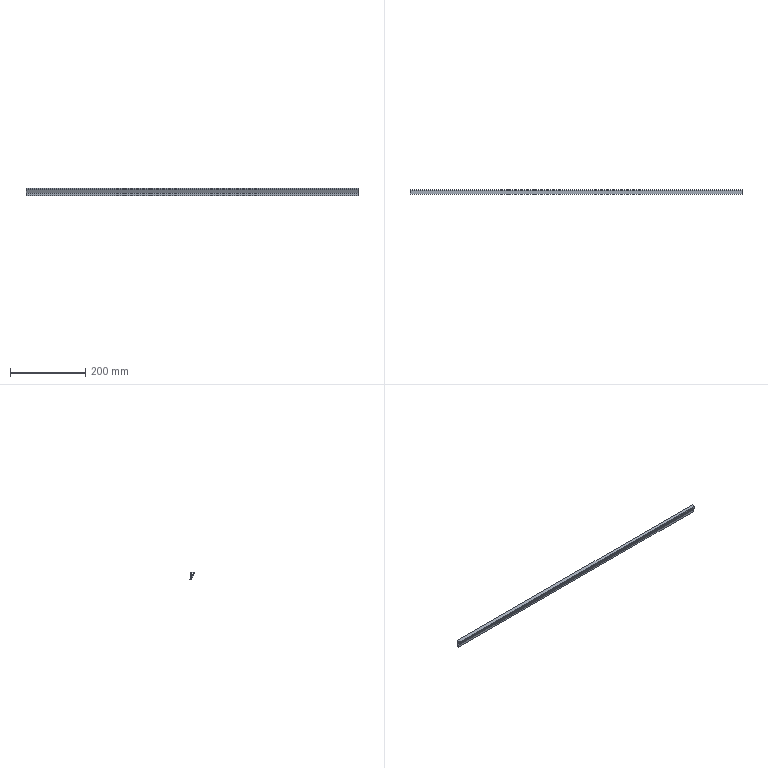Part | SolidWorks | features BaseBody 1 | 1 solid | 13 faces | box 880 x 12 x 21 mm | volume 96538 mm3 | plane 13
STEP:
#1=CARTESIAN_POINT('',(440.,0.,0.));
#2=VERTEX_POINT('',#1);
#3=CARTESIAN_POINT('',(-440.,0.,0.));
#4=VERTEX_POINT('',#3);
#5=CARTESIAN_POINT('',(440.,0.,0.));
#6=DIRECTION('',(-1.,0.,0.));
#7=VECTOR('',#6,1000.);
#8=LINE('',#5,#7);
#9=EDGE_CURVE('',#2,#4,#8,.T.);
#10=ORIENTED_EDGE('',*,*,#9,.F.);
#11=CARTESIAN_POINT('',(440.,0.,-19.));
#12=VERTEX_POINT('',#11);
#13=CARTESIAN_POINT('',(440.,0.,-19.));
#14=DIRECTION('',(0.,0.,1.));
#15=VECTOR('',#14,1000.);
#16=LINE('',#13,#15);
#17=EDGE_CURVE('',#12,#2,#16,.T.);
#18=ORIENTED_EDGE('',*,*,#17,.F.);
#19=CARTESIAN_POINT('',(-440.,0.,-19.));
#20=VERTEX_POINT('',#19);
#21=CARTESIAN_POINT('',(440.,0.,-19.));
#22=DIRECTION('',(1.,0.,0.));
#23=VECTOR('',#22,1000.);
#24=LINE('',#21,#23);
#25=EDGE_CURVE('',#20,#12,#24,.T.);
#26=ORIENTED_EDGE('',*,*,#25,.F.);
#27=CARTESIAN_POINT('',(-440.,0.,-19.));
#28=DIRECTION('',(0.,0.,-1.));
#29=VECTOR('',#28,1000.);
#30=LINE('',#27,#29);
#31=EDGE_CURVE('',#4,#20,#30,.T.);
#32=ORIENTED_EDGE('',*,*,#31,.F.);
#33=EDGE_LOOP('',(#10,#18,#26,#32));
#34=FACE_OUTER_BOUND('',#33,.T.);
#35=CARTESIAN_POINT('',(440.,0.,-19.));
#36=DIRECTION('',(0.,-1.,0.));
#37=DIRECTION('',(0.,0.,-1.));
#38=AXIS2_PLACEMENT_3D('',#35,#36,#37);
#39=PLANE('',#38);
#40=ADVANCED_FACE('',(#34),#39,.F.);
#41=CARTESIAN_POINT('',(-440.,-3.,-3.));
#42=VERTEX_POINT('',#41);
#43=CARTESIAN_POINT('',(-440.,-3.,-21.));
#44=VERTEX_POINT('',#43);
#45=CARTESIAN_POINT('',(-440.,-3.,0.));
#46=DIRECTION('',(0.,0.,-1.));
#47=VECTOR('',#46,1000.);
#48=LINE('',#45,#47);
#49=EDGE_CURVE('',#42,#44,#48,.T.);
#50=ORIENTED_EDGE('',*,*,#49,.F.);
#51=CARTESIAN_POINT('',(-440.,-7.,-3.));
#52=VERTEX_POINT('',#51);
#53=CARTESIAN_POINT('',(-440.,0.,-3.));
#54=DIRECTION('',(0.,1.,0.));
#55=VECTOR('',#54,1000.);
#56=LINE('',#53,#55);
#57=EDGE_CURVE('',#52,#42,#56,.T.);
#58=ORIENTED_EDGE('',*,*,#57,.F.);
#59=CARTESIAN_POINT('',(-440.,-5.,-7.134));
#60=VERTEX_POINT('',#59);
#61=CARTESIAN_POINT('',(-440.,-5.,-7.134));
#62=DIRECTION('',(0.,-0.4355,0.9002));
#63=VECTOR('',#62,1000.);
#64=LINE('',#61,#63);
#65=EDGE_CURVE('',#60,#52,#64,.T.);
#66=ORIENTED_EDGE('',*,*,#65,.F.);
#67=CARTESIAN_POINT('',(-440.,-5.,-13.334));
#68=VERTEX_POINT('',#67);
#69=CARTESIAN_POINT('',(-440.,-5.,0.));
#70=DIRECTION('',(0.,0.,1.));
#71=VECTOR('',#70,1000.);
#72=LINE('',#69,#71);
#73=EDGE_CURVE('',#68,#60,#72,.T.);
#74=ORIENTED_EDGE('',*,*,#73,.F.);
#75=CARTESIAN_POINT('',(-440.,-10.,-3.));
#76=VERTEX_POINT('',#75);
#77=CARTESIAN_POINT('',(-440.,-10.,-3.));
#78=DIRECTION('',(0.,0.4355,-0.9002));
#79=VECTOR('',#78,1000.);
#80=LINE('',#77,#79);
#81=EDGE_CURVE('',#76,#68,#80,.T.);
#82=ORIENTED_EDGE('',*,*,#81,.F.);
#83=CARTESIAN_POINT('',(-440.,-10.,0.));
#84=VERTEX_POINT('',#83);
#85=CARTESIAN_POINT('',(-440.,-10.,0.));
#86=DIRECTION('',(0.,0.,-1.));
#87=VECTOR('',#86,1000.);
#88=LINE('',#85,#87);
#89=EDGE_CURVE('',#84,#76,#88,.T.);
#90=ORIENTED_EDGE('',*,*,#89,.F.);
#91=CARTESIAN_POINT('',(-440.,0.,0.));
#92=DIRECTION('',(0.,-1.,0.));
#93=VECTOR('',#92,1000.);
#94=LINE('',#91,#93);
#95=EDGE_CURVE('',#4,#84,#94,.T.);
#96=ORIENTED_EDGE('',*,*,#95,.F.);
#97=ORIENTED_EDGE('',*,*,#31,.T.);
#98=CARTESIAN_POINT('',(-440.,2.,-19.));
#99=VERTEX_POINT('',#98);
#100=CARTESIAN_POINT('',(-440.,0.,-19.));
#101=DIRECTION('',(0.,-1.,0.));
#102=VECTOR('',#101,1000.);
#103=LINE('',#100,#102);
#104=EDGE_CURVE('',#99,#20,#103,.T.);
#105=ORIENTED_EDGE('',*,*,#104,.F.);
#106=CARTESIAN_POINT('',(-440.,2.,-21.));
#107=VERTEX_POINT('',#106);
#108=CARTESIAN_POINT('',(-440.,2.,0.));
#109=DIRECTION('',(0.,0.,1.));
#110=VECTOR('',#109,1000.);
#111=LINE('',#108,#110);
#112=EDGE_CURVE('',#107,#99,#111,.T.);
#113=ORIENTED_EDGE('',*,*,#112,.F.);
#114=CARTESIAN_POINT('',(-440.,0.,-21.));
#115=DIRECTION('',(0.,1.,0.));
#116=VECTOR('',#115,1000.);
#117=LINE('',#114,#116);
#118=EDGE_CURVE('',#44,#107,#117,.T.);
#119=ORIENTED_EDGE('',*,*,#118,.F.);
#120=EDGE_LOOP('',(#50,#58,#66,#74,#82,#90,#96,#97,#105,#113,#119));
#121=FACE_OUTER_BOUND('',#120,.T.);
#122=CARTESIAN_POINT('',(-440.,0.,0.));
#123=DIRECTION('',(1.,0.,0.));
#124=DIRECTION('',(0.,0.,-1.));
#125=AXIS2_PLACEMENT_3D('',#122,#123,#124);
#126=PLANE('',#125);
#127=ADVANCED_FACE('',(#121),#126,.F.);
#128=CARTESIAN_POINT('',(440.,-10.,0.));
#129=VERTEX_POINT('',#128);
#130=CARTESIAN_POINT('',(440.,-10.,0.));
#131=DIRECTION('',(-1.,0.,0.));
#132=VECTOR('',#131,1000.);
#133=LINE('',#130,#132);
#134=EDGE_CURVE('',#129,#84,#133,.T.);
#135=ORIENTED_EDGE('',*,*,#134,.F.);
#136=CARTESIAN_POINT('',(440.,0.,0.));
#137=DIRECTION('',(0.,-1.,0.));
#138=VECTOR('',#137,1000.);
#139=LINE('',#136,#138);
#140=EDGE_CURVE('',#2,#129,#139,.T.);
#141=ORIENTED_EDGE('',*,*,#140,.F.);
#142=ORIENTED_EDGE('',*,*,#9,.T.);
#143=ORIENTED_EDGE('',*,*,#95,.T.);
#144=EDGE_LOOP('',(#135,#141,#142,#143));
#145=FACE_OUTER_BOUND('',#144,.T.);
#146=CARTESIAN_POINT('',(440.,0.,0.));
#147=DIRECTION('',(0.,0.,-1.));
#148=DIRECTION('',(-1.,0.,0.));
#149=AXIS2_PLACEMENT_3D('',#146,#147,#148);
#150=PLANE('',#149);
#151=ADVANCED_FACE('',(#145),#150,.F.);
#152=CARTESIAN_POINT('',(440.,-7.,-3.));
#153=VERTEX_POINT('',#152);
#154=CARTESIAN_POINT('',(440.,-3.,-3.));
#155=VERTEX_POINT('',#154);
#156=CARTESIAN_POINT('',(440.,0.,-3.));
#157=DIRECTION('',(0.,1.,0.));
#158=VECTOR('',#157,1000.);
#159=LINE('',#156,#158);
#160=EDGE_CURVE('',#153,#155,#159,.T.);
#161=ORIENTED_EDGE('',*,*,#160,.T.);
#162=CARTESIAN_POINT('',(440.,-3.,-21.));
#163=VERTEX_POINT('',#162);
#164=CARTESIAN_POINT('',(440.,-3.,0.));
#165=DIRECTION('',(0.,0.,-1.));
#166=VECTOR('',#165,1000.);
#167=LINE('',#164,#166);
#168=EDGE_CURVE('',#155,#163,#167,.T.);
#169=ORIENTED_EDGE('',*,*,#168,.T.);
#170=CARTESIAN_POINT('',(440.,2.,-21.));
#171=VERTEX_POINT('',#170);
#172=CARTESIAN_POINT('',(440.,0.,-21.));
#173=DIRECTION('',(0.,1.,0.));
#174=VECTOR('',#173,1000.);
#175=LINE('',#172,#174);
#176=EDGE_CURVE('',#163,#171,#175,.T.);
#177=ORIENTED_EDGE('',*,*,#176,.T.);
#178=CARTESIAN_POINT('',(440.,2.,-19.));
#179=VERTEX_POINT('',#178);
#180=CARTESIAN_POINT('',(440.,2.,0.));
#181=DIRECTION('',(0.,0.,1.));
#182=VECTOR('',#181,1000.);
#183=LINE('',#180,#182);
#184=EDGE_CURVE('',#171,#179,#183,.T.);
#185=ORIENTED_EDGE('',*,*,#184,.T.);
#186=CARTESIAN_POINT('',(440.,0.,-19.));
#187=DIRECTION('',(0.,-1.,0.));
#188=VECTOR('',#187,1000.);
#189=LINE('',#186,#188);
#190=EDGE_CURVE('',#179,#12,#189,.T.);
#191=ORIENTED_EDGE('',*,*,#190,.T.);
#192=ORIENTED_EDGE('',*,*,#17,.T.);
#193=ORIENTED_EDGE('',*,*,#140,.T.);
#194=CARTESIAN_POINT('',(440.,-10.,-3.));
#195=VERTEX_POINT('',#194);
#196=CARTESIAN_POINT('',(440.,-10.,0.));
#197=DIRECTION('',(0.,0.,-1.));
#198=VECTOR('',#197,1000.);
#199=LINE('',#196,#198);
#200=EDGE_CURVE('',#129,#195,#199,.T.);
#201=ORIENTED_EDGE('',*,*,#200,.T.);
#202=CARTESIAN_POINT('',(440.,-5.,-13.334));
#203=VERTEX_POINT('',#202);
#204=CARTESIAN_POINT('',(440.,-10.,-3.));
#205=DIRECTION('',(0.,0.4355,-0.9002));
#206=VECTOR('',#205,1000.);
#207=LINE('',#204,#206);
#208=EDGE_CURVE('',#195,#203,#207,.T.);
#209=ORIENTED_EDGE('',*,*,#208,.T.);
#210=CARTESIAN_POINT('',(440.,-5.,-7.134));
#211=VERTEX_POINT('',#210);
#212=CARTESIAN_POINT('',(440.,-5.,0.));
#213=DIRECTION('',(0.,0.,1.));
#214=VECTOR('',#213,1000.);
#215=LINE('',#212,#214);
#216=EDGE_CURVE('',#203,#211,#215,.T.);
#217=ORIENTED_EDGE('',*,*,#216,.T.);
#218=CARTESIAN_POINT('',(440.,-5.,-7.134));
#219=DIRECTION('',(0.,-0.4355,0.9002));
#220=VECTOR('',#219,1000.);
#221=LINE('',#218,#220);
#222=EDGE_CURVE('',#211,#153,#221,.T.);
#223=ORIENTED_EDGE('',*,*,#222,.T.);
#224=EDGE_LOOP('',(#161,#169,#177,#185,#191,#192,#193,#201,#209,#217,#223));
#225=FACE_OUTER_BOUND('',#224,.T.);
#226=CARTESIAN_POINT('',(440.,0.,0.));
#227=DIRECTION('',(1.,0.,0.));
#228=DIRECTION('',(0.,0.,-1.));
#229=AXIS2_PLACEMENT_3D('',#226,#227,#228);
#230=PLANE('',#229);
#231=ADVANCED_FACE('',(#225),#230,.T.);
#232=ORIENTED_EDGE('',*,*,#25,.T.);
#233=ORIENTED_EDGE('',*,*,#190,.F.);
#234=CARTESIAN_POINT('',(440.,2.,-19.));
#235=DIRECTION('',(1.,0.,0.));
#236=VECTOR('',#235,1000.);
#237=LINE('',#234,#236);
#238=EDGE_CURVE('',#99,#179,#237,.T.);
#239=ORIENTED_EDGE('',*,*,#238,.F.);
#240=ORIENTED_EDGE('',*,*,#104,.T.);
#241=EDGE_LOOP('',(#232,#233,#239,#240));
#242=FACE_OUTER_BOUND('',#241,.T.);
#243=CARTESIAN_POINT('',(440.,2.,-19.));
#244=DIRECTION('',(0.,0.,-1.));
#245=DIRECTION('',(-1.,0.,0.));
#246=AXIS2_PLACEMENT_3D('',#243,#244,#245);
#247=PLANE('',#246);
#248=ADVANCED_FACE('',(#242),#247,.F.);
#249=CARTESIAN_POINT('',(440.,2.,-21.));
#250=DIRECTION('',(-1.,0.,0.));
#251=VECTOR('',#250,1000.);
#252=LINE('',#249,#251);
#253=EDGE_CURVE('',#171,#107,#252,.T.);
#254=ORIENTED_EDGE('',*,*,#253,.F.);
#255=ORIENTED_EDGE('',*,*,#176,.F.);
#256=CARTESIAN_POINT('',(440.,-3.,-21.));
#257=DIRECTION('',(1.,0.,0.));
#258=VECTOR('',#257,1000.);
#259=LINE('',#256,#258);
#260=EDGE_CURVE('',#44,#163,#259,.T.);
#261=ORIENTED_EDGE('',*,*,#260,.F.);
#262=ORIENTED_EDGE('',*,*,#118,.T.);
#263=EDGE_LOOP('',(#254,#255,#261,#262));
#264=FACE_OUTER_BOUND('',#263,.T.);
#265=CARTESIAN_POINT('',(440.,2.,-21.));
#266=DIRECTION('',(0.,0.,1.));
#267=DIRECTION('',(1.,0.,0.));
#268=AXIS2_PLACEMENT_3D('',#265,#266,#267);
#269=PLANE('',#268);
#270=ADVANCED_FACE('',(#264),#269,.F.);
#271=ORIENTED_EDGE('',*,*,#260,.T.);
#272=ORIENTED_EDGE('',*,*,#168,.F.);
#273=CARTESIAN_POINT('',(440.,-3.,-3.));
#274=DIRECTION('',(1.,0.,0.));
#275=VECTOR('',#274,1000.);
#276=LINE('',#273,#275);
#277=EDGE_CURVE('',#42,#155,#276,.T.);
#278=ORIENTED_EDGE('',*,*,#277,.F.);
#279=ORIENTED_EDGE('',*,*,#49,.T.);
#280=EDGE_LOOP('',(#271,#272,#278,#279));
#281=FACE_OUTER_BOUND('',#280,.T.);
#282=CARTESIAN_POINT('',(440.,-3.,-3.));
#283=DIRECTION('',(0.,1.,0.));
#284=DIRECTION('',(0.,0.,1.));
#285=AXIS2_PLACEMENT_3D('',#282,#283,#284);
#286=PLANE('',#285);
#287=ADVANCED_FACE('',(#281),#286,.F.);
#288=ORIENTED_EDGE('',*,*,#277,.T.);
#289=ORIENTED_EDGE('',*,*,#160,.F.);
#290=CARTESIAN_POINT('',(440.,-7.,-3.));
#291=DIRECTION('',(1.,0.,0.));
#292=VECTOR('',#291,1000.);
#293=LINE('',#290,#292);
#294=EDGE_CURVE('',#52,#153,#293,.T.);
#295=ORIENTED_EDGE('',*,*,#294,.F.);
#296=ORIENTED_EDGE('',*,*,#57,.T.);
#297=EDGE_LOOP('',(#288,#289,#295,#296));
#298=FACE_OUTER_BOUND('',#297,.T.);
#299=CARTESIAN_POINT('',(440.,-7.,-3.));
#300=DIRECTION('',(0.,0.,1.));
#301=DIRECTION('',(1.,0.,0.));
#302=AXIS2_PLACEMENT_3D('',#299,#300,#301);
#303=PLANE('',#302);
#304=ADVANCED_FACE('',(#298),#303,.F.);
#305=ORIENTED_EDGE('',*,*,#294,.T.);
#306=ORIENTED_EDGE('',*,*,#222,.F.);
#307=CARTESIAN_POINT('',(440.,-5.,-7.134));
#308=DIRECTION('',(1.,0.,0.));
#309=VECTOR('',#308,1000.);
#310=LINE('',#307,#309);
#311=EDGE_CURVE('',#60,#211,#310,.T.);
#312=ORIENTED_EDGE('',*,*,#311,.F.);
#313=ORIENTED_EDGE('',*,*,#65,.T.);
#314=EDGE_LOOP('',(#305,#306,#312,#313));
#315=FACE_OUTER_BOUND('',#314,.T.);
#316=CARTESIAN_POINT('',(440.,-5.,-7.134));
#317=DIRECTION('',(0.,-0.9002,-0.4355));
#318=DIRECTION('',(0.,0.4355,-0.9002));
#319=AXIS2_PLACEMENT_3D('',#316,#317,#318);
#320=PLANE('',#319);
#321=ADVANCED_FACE('',(#315),#320,.F.);
#322=ORIENTED_EDGE('',*,*,#311,.T.);
#323=ORIENTED_EDGE('',*,*,#216,.F.);
#324=CARTESIAN_POINT('',(440.,-5.,-13.334));
#325=DIRECTION('',(1.,0.,0.));
#326=VECTOR('',#325,1000.);
#327=LINE('',#324,#326);
#328=EDGE_CURVE('',#68,#203,#327,.T.);
#329=ORIENTED_EDGE('',*,*,#328,.F.);
#330=ORIENTED_EDGE('',*,*,#73,.T.);
#331=EDGE_LOOP('',(#322,#323,#329,#330));
#332=FACE_OUTER_BOUND('',#331,.T.);
#333=CARTESIAN_POINT('',(440.,-5.,-13.334));
#334=DIRECTION('',(0.,-1.,0.));
#335=DIRECTION('',(0.,0.,-1.));
#336=AXIS2_PLACEMENT_3D('',#333,#334,#335);
#337=PLANE('',#336);
#338=ADVANCED_FACE('',(#332),#337,.F.);
#339=ORIENTED_EDGE('',*,*,#328,.T.);
#340=ORIENTED_EDGE('',*,*,#208,.F.);
#341=CARTESIAN_POINT('',(440.,-10.,-3.));
#342=DIRECTION('',(1.,0.,0.));
#343=VECTOR('',#342,1000.);
#344=LINE('',#341,#343);
#345=EDGE_CURVE('',#76,#195,#344,.T.);
#346=ORIENTED_EDGE('',*,*,#345,.F.);
#347=ORIENTED_EDGE('',*,*,#81,.T.);
#348=EDGE_LOOP('',(#339,#340,#346,#347));
#349=FACE_OUTER_BOUND('',#348,.T.);
#350=CARTESIAN_POINT('',(440.,-7.795,-7.557));
#351=DIRECTION('',(0.,0.9002,0.4355));
#352=DIRECTION('',(0.,-0.4355,0.9002));
#353=AXIS2_PLACEMENT_3D('',#350,#351,#352);
#354=PLANE('',#353);
#355=ADVANCED_FACE('',(#349),#354,.F.);
#356=ORIENTED_EDGE('',*,*,#345,.T.);
#357=ORIENTED_EDGE('',*,*,#200,.F.);
#358=ORIENTED_EDGE('',*,*,#134,.T.);
#359=ORIENTED_EDGE('',*,*,#89,.T.);
#360=EDGE_LOOP('',(#356,#357,#358,#359));
#361=FACE_OUTER_BOUND('',#360,.T.);
#362=CARTESIAN_POINT('',(440.,-10.,0.));
#363=DIRECTION('',(0.,1.,0.));
#364=DIRECTION('',(0.,0.,1.));
#365=AXIS2_PLACEMENT_3D('',#362,#363,#364);
#366=PLANE('',#365);
#367=ADVANCED_FACE('',(#361),#366,.F.);
#368=ORIENTED_EDGE('',*,*,#238,.T.);
#369=ORIENTED_EDGE('',*,*,#184,.F.);
#370=ORIENTED_EDGE('',*,*,#253,.T.);
#371=ORIENTED_EDGE('',*,*,#112,.T.);
#372=EDGE_LOOP('',(#368,#369,#370,#371));
#373=FACE_OUTER_BOUND('',#372,.T.);
#374=CARTESIAN_POINT('',(440.,2.,-21.));
#375=DIRECTION('',(0.,-1.,0.));
#376=DIRECTION('',(0.,0.,-1.));
#377=AXIS2_PLACEMENT_3D('',#374,#375,#376);
#378=PLANE('',#377);
#379=ADVANCED_FACE('',(#373),#378,.F.);
#380=CLOSED_SHELL('',(#40,#127,#151,#231,#248,#270,#287,#304,#321,#338,#355,#367,#379));
#381=MANIFOLD_SOLID_BREP('',#380);
#382=CARTESIAN_POINT('',(0.,0.,0.));
#383=DIRECTION('',(0.,0.,1.));
#384=DIRECTION('',(1.,0.,0.));
#385=AXIS2_PLACEMENT_3D('',#382,#383,#384);
#386=(LENGTH_UNIT()NAMED_UNIT(*)SI_UNIT(.MILLI.,.METRE.));
#387=UNCERTAINTY_MEASURE_WITH_UNIT(LENGTH_MEASURE(0.00001),#386,'','');
#388=(NAMED_UNIT(*)PLANE_ANGLE_UNIT()SI_UNIT($,.RADIAN.));
#389=(NAMED_UNIT(*)SI_UNIT($,.STERADIAN.)SOLID_ANGLE_UNIT());
#390=(GEOMETRIC_REPRESENTATION_CONTEXT(3)GLOBAL_UNCERTAINTY_ASSIGNED_CONTEXT((#387))GLOBAL_UNIT_ASSIGNED_CONTEXT((#386,#388,#389))REPRESENTATION_CONTEXT('',''));
#391=ADVANCED_BREP_SHAPE_REPRESENTATION('',(#381,#385),#390);